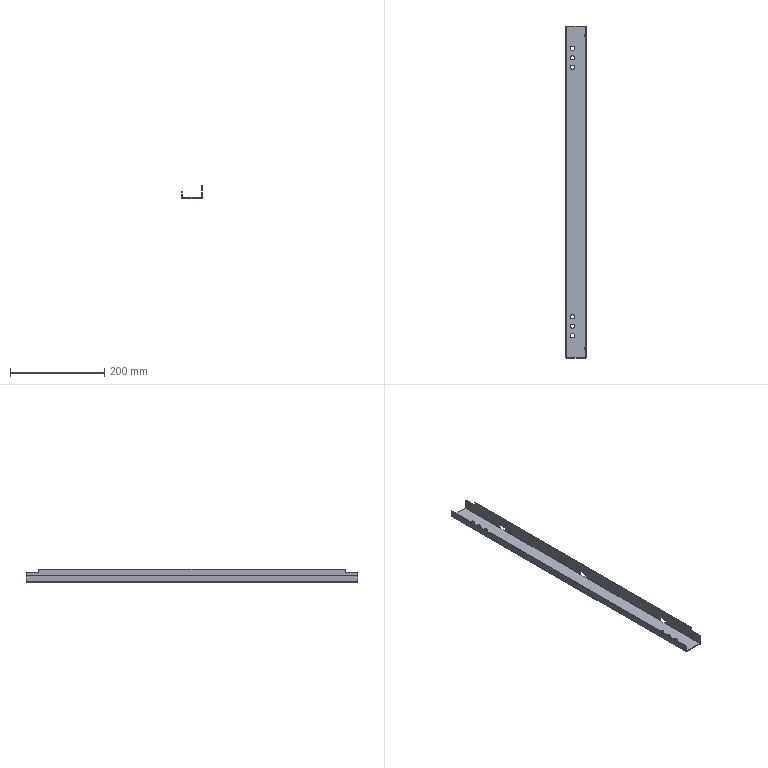Part | STEP file | Lower door gasket strip vertical (hinge) modified | 1 solid | 88 faces | box 44.5 x 705 x 28.5 mm | volume 113772 mm3 | plane 62 | cylinder 26 | commonest cylinder face diameters 9 x12 1 x7 5 x7